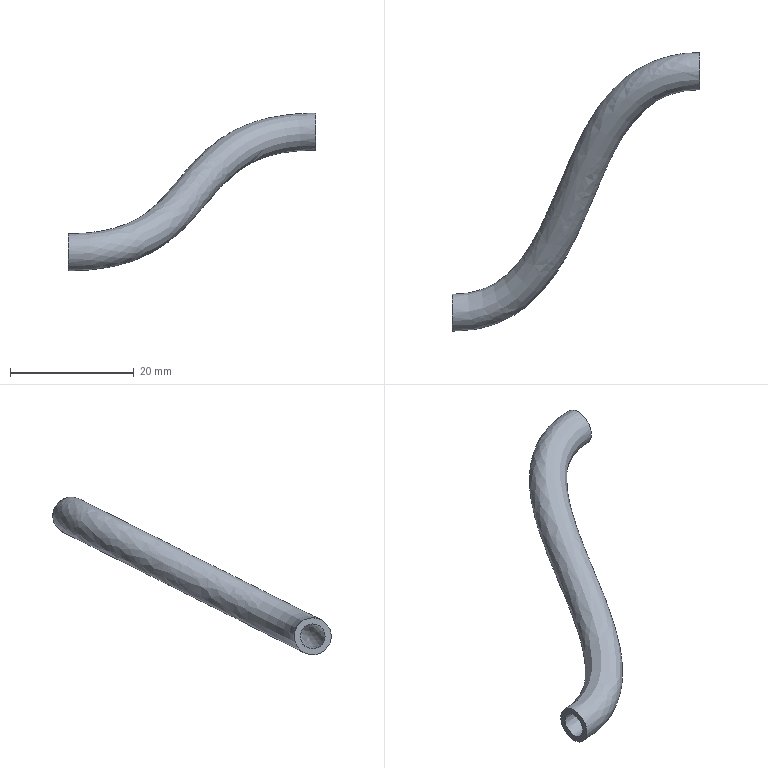Part | NX | features solid 2 | 1 solid | 4 faces | box 40.058 x 45.002 x 25.5 mm | volume 999.442 mm3 | plane 2 | spline 2